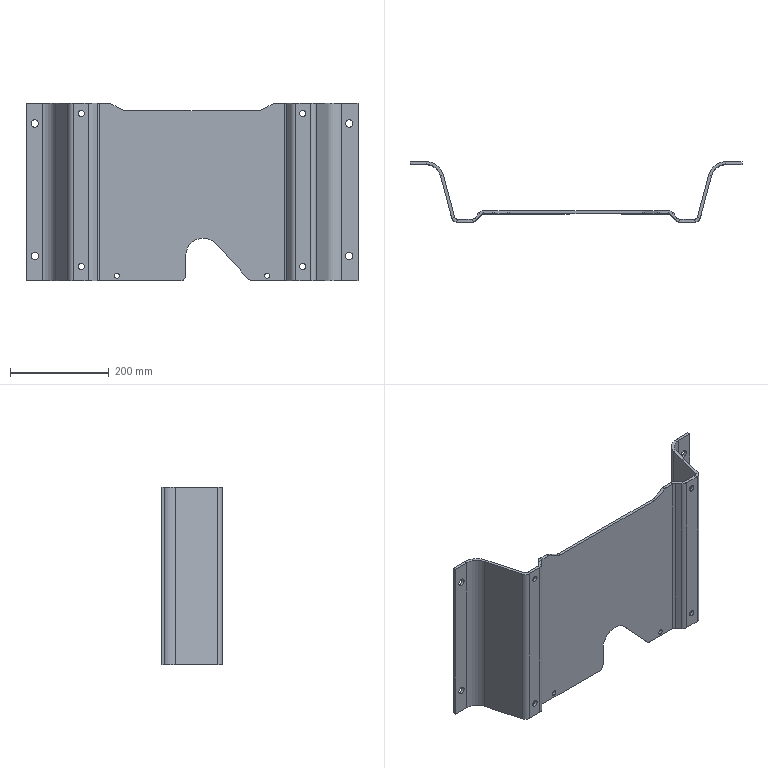Part | SolidWorks | features Fillet 2, ICE 2, FlatPattern 1, SMBaseFlange 1, SheetMetal 1 | 1 solid | 105 faces | box 674 x 122.8 x 360 mm | volume 1751347 mm3 | plane 61 | cylinder 44 | commonest cylinder face diameters 12.5 x8 15 x8 12 x6 20 x6 24 x6 10 x4